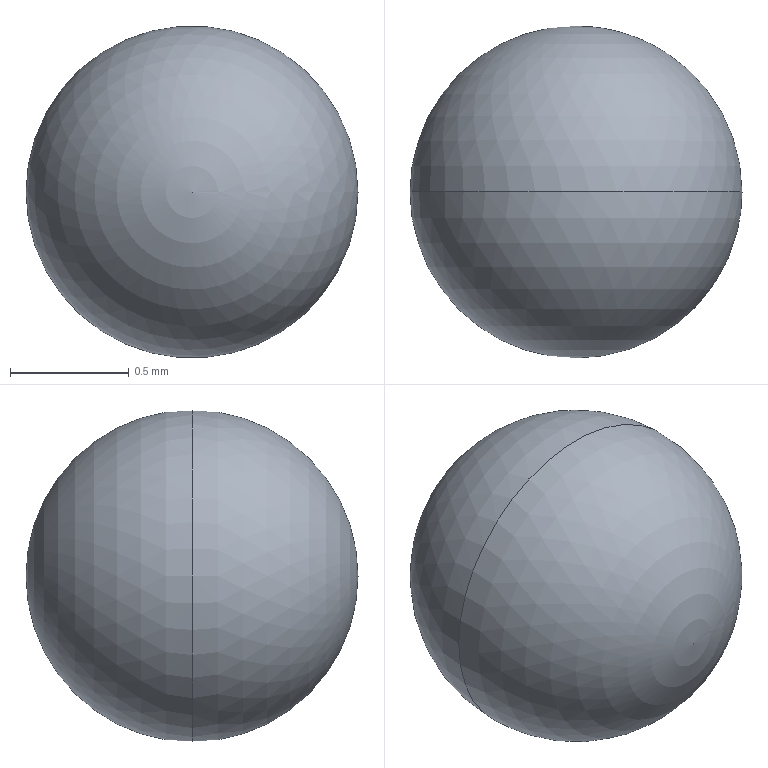Part | NX | 1 solid | 2 faces | box 1.4 x 1.4 x 1.4 mm | volume 1.437 mm3 | sphere 2
STEP:
#1=CARTESIAN_POINT('',(-12.15,0.,26.));
#2=VERTEX_POINT('',#1);
#3=CARTESIAN_POINT('',(-13.55,0.,26.));
#4=VERTEX_POINT('',#3);
#5=CARTESIAN_POINT('',(-12.85,0.,26.));
#6=DIRECTION('',(0.,1.,0.));
#7=DIRECTION('',(1.,0.,0.));
#8=AXIS2_PLACEMENT_3D('',#5,#6,#7);
#9=CIRCLE('',#8,0.7);
#10=EDGE_CURVE('',#2,#4,#9,.T.);
#11=ORIENTED_EDGE('',*,*,#10,.T.);
#12=CARTESIAN_POINT('',(-12.85,0.,26.));
#13=DIRECTION('',(0.,1.,0.));
#14=DIRECTION('',(1.,0.,0.));
#15=AXIS2_PLACEMENT_3D('',#12,#13,#14);
#16=CIRCLE('',#15,0.7);
#17=EDGE_CURVE('',#4,#2,#16,.T.);
#18=ORIENTED_EDGE('',*,*,#17,.T.);
#19=EDGE_LOOP('',(#11,#18));
#20=FACE_BOUND('',#19,.T.);
#21=CARTESIAN_POINT('',(-12.85,0.,26.));
#22=DIRECTION('',(0.,1.,0.));
#23=DIRECTION('',(1.,0.,0.));
#24=AXIS2_PLACEMENT_3D('',#21,#22,#23);
#25=SPHERICAL_SURFACE('',#24,0.7);
#26=ADVANCED_FACE('',(#20),#25,.T.);
#27=ORIENTED_EDGE('',*,*,#10,.F.);
#28=ORIENTED_EDGE('',*,*,#17,.F.);
#29=EDGE_LOOP('',(#27,#28));
#30=FACE_BOUND('',#29,.T.);
#31=CARTESIAN_POINT('',(-12.85,0.,26.));
#32=DIRECTION('',(0.,1.,0.));
#33=DIRECTION('',(1.,0.,0.));
#34=AXIS2_PLACEMENT_3D('',#31,#32,#33);
#35=SPHERICAL_SURFACE('',#34,0.7);
#36=ADVANCED_FACE('',(#30),#35,.T.);
#37=CLOSED_SHELL('',(#26,#36));
#38=MANIFOLD_SOLID_BREP('',#37);
#39=(LENGTH_UNIT()NAMED_UNIT(*)SI_UNIT(.MILLI.,.METRE.));
#40=UNCERTAINTY_MEASURE_WITH_UNIT(LENGTH_MEASURE(0.00001),#39,'','');
#41=(NAMED_UNIT(*)PLANE_ANGLE_UNIT()SI_UNIT($,.RADIAN.));
#42=(NAMED_UNIT(*)SI_UNIT($,.STERADIAN.)SOLID_ANGLE_UNIT());
#43=(GEOMETRIC_REPRESENTATION_CONTEXT(3)GLOBAL_UNCERTAINTY_ASSIGNED_CONTEXT((#40))GLOBAL_UNIT_ASSIGNED_CONTEXT((#39,#41,#42))REPRESENTATION_CONTEXT('',''));
#44=ADVANCED_BREP_SHAPE_REPRESENTATION('',(#38),#43);